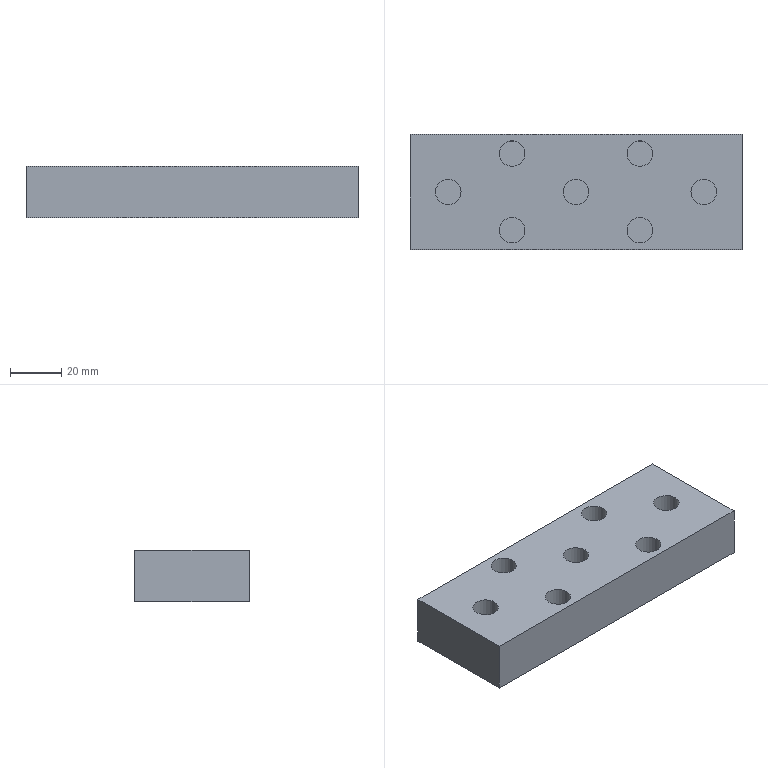NC program | NX | posted with a generic post | part box 130 x 45 x 20 mm
Lines 288 to 1135 of 3690:
(PLANAR_MILL_1 , TOOL : D8开粗)
N556 T09 M6
N558 G54
N560 G17 G0 G90 X-25.452 Y14.224 S4500 M3
N562 G43 Z30. H9
N564 Z1.
N566 G94 G1 X-25.239 Y14.101 Z0.987 F800.
N568 X-24.753 Y14.103 Z0.962
N570 X-24.347 Y14.338 Z0.937
N572 X-24.1 Y14.766 Z0.911
N574 Y15.234 Z0.887
N576 X-24.347 Y15.662 Z0.861
N578 X-24.753 Y15.897 Z0.836
N580 X-25.239 Y15.899 Z0.811
N582 X-25.659 Y15.656 Z0.785
N584 X-25.9 Y15.234 Z0.76
N586 Y14.766 Z0.735
N588 X-25.659 Y14.344 Z0.71
N590 X-25.239 Y14.101 Z0.684
N592 X-24.753 Y14.103 Z0.659
N594 X-24.347 Y14.338 Z0.634
N596 X-24.1 Y14.766 Z0.608
N598 Y15.234 Z0.584
N600 X-24.347 Y15.662 Z0.558
N602 X-24.753 Y15.897 Z0.533
N604 X-25.239 Y15.899 Z0.508
N606 X-25.659 Y15.656 Z0.483
N608 X-25.9 Y15.234 Z0.457
N610 Y14.766 Z0.432
N612 X-25.659 Y14.344 Z0.407
N614 X-25.239 Y14.101 Z0.382
N616 X-24.753 Y14.103 Z0.356
N618 X-24.347 Y14.338 Z0.332
N620 X-24.1 Y14.766 Z0.306
N622 Y15.234 Z0.281
N624 X-24.347 Y15.662 Z0.255
N626 X-24.753 Y15.897 Z0.231
N628 X-25.239 Y15.899 Z0.205
N630 X-25.659 Y15.656 Z0.18
N632 X-25.9 Y15.234 Z0.154
N634 Y14.766 Z0.13
N636 X-25.659 Y14.344 Z0.104
N638 X-25.239 Y14.101 Z0.079
N640 X-24.753 Y14.103 Z0.053
N642 X-24.347 Y14.338 Z0.029
N644 X-24.1 Y14.766 Z0.003
N646 Y15.234 Z-0.022
N648 X-24.347 Y15.662 Z-0.048
N650 X-24.753 Y15.897 Z-0.072
N652 X-25.239 Y15.899 Z-0.098
N654 X-25.659 Y15.656 Z-0.123
N656 X-25.9 Y15.234 Z-0.148
N658 Y14.766 Z-0.173
N660 X-25.659 Y14.344 Z-0.198
N662 X-25.239 Y14.101 Z-0.224
N664 X-24.753 Y14.103 Z-0.249
N666 X-24.347 Y14.338 Z-0.274
N668 X-24.1 Y14.766 Z-0.3
N670 Y15.234 Z-0.324
N672 X-24.347 Y15.662 Z-0.35
N674 X-24.753 Y15.897 Z-0.375
N676 X-25.239 Y15.899 Z-0.4
N678 X-25.659 Y15.656 Z-0.426
N680 X-25.9 Y15.234 Z-0.451
N682 Y14.766 Z-0.476
N684 X-25.659 Y14.344 Z-0.501
N686 X-25.239 Y14.101 Z-0.527
N688 X-24.753 Y14.103 Z-0.552
N690 X-24.347 Y14.338 Z-0.577
N692 X-24.1 Y14.766 Z-0.603
N694 Y15.234 Z-0.627
N696 X-24.347 Y15.662 Z-0.653
N698 X-24.753 Y15.897 Z-0.678
N700 X-25.239 Y15.899 Z-0.703
N702 X-25.659 Y15.656 Z-0.728
N704 X-25.9 Y15.234 Z-0.754
N706 Y14.766 Z-0.778
N708 X-25.659 Y14.344 Z-0.804
N710 X-25.239 Y14.101 Z-0.829
N712 X-24.753 Y14.103 Z-0.855
N714 X-24.347 Y14.338 Z-0.879
N716 X-24.1 Y14.766 Z-0.905
N718 Y15.234 Z-0.93
N720 X-24.347 Y15.662 Z-0.956
N722 X-24.753 Y15.897 Z-0.98
N724 X-25.239 Y15.899 Z-1.006
N726 X-25.659 Y15.656 Z-1.031
N728 X-25.9 Y15.234 Z-1.057
N730 Y14.766 Z-1.081
N732 X-25.659 Y14.344 Z-1.107
N734 X-25.239 Y14.101 Z-1.132
N736 X-24.753 Y14.103 Z-1.158
N738 X-24.347 Y14.338 Z-1.182
N740 X-24.1 Y14.766 Z-1.208
N742 Y15.234 Z-1.233
N744 X-24.347 Y15.662 Z-1.259
N746 X-24.753 Y15.897 Z-1.283
N748 X-25.239 Y15.899 Z-1.309
N750 X-25.659 Y15.656 Z-1.334
N752 X-25.9 Y15.234 Z-1.359
N754 Y14.766 Z-1.384
N756 X-25.659 Y14.344 Z-1.409
N758 X-25.239 Y14.101 Z-1.435
N760 X-24.753 Y14.103 Z-1.46
N762 X-24.347 Y14.338 Z-1.485
N764 X-24.1 Y14.766 Z-1.511
N766 Y15.234 Z-1.535
N768 X-24.347 Y15.662 Z-1.561
N770 X-24.753 Y15.897 Z-1.586
N772 X-25.239 Y15.899 Z-1.611
N774 X-25.659 Y15.656 Z-1.637
N776 X-25.9 Y15.234 Z-1.662
N778 Y14.766 Z-1.687
N780 X-25.659 Y14.344 Z-1.712
N782 X-25.239 Y14.101 Z-1.738
N784 X-24.753 Y14.103 Z-1.763
N786 X-24.347 Y14.338 Z-1.788
N788 X-24.1 Y14.766 Z-1.814
N790 Y15.234 Z-1.838
N792 X-24.347 Y15.662 Z-1.864
N794 X-24.753 Y15.897 Z-1.889
N796 X-25.239 Y15.899 Z-1.914
N798 X-25.659 Y15.656 Z-1.939
N800 X-25.9 Y15.234 Z-1.965
N802 Y14.766 Z-1.989
N804 X-25.659 Y14.344 Z-2.015
N806 X-25.239 Y14.101 Z-2.04
N808 X-24.753 Y14.103 Z-2.066
N810 X-24.347 Y14.338 Z-2.09
N812 X-24.1 Y14.766 Z-2.116
N814 Y15.234 Z-2.141
N816 X-24.347 Y15.662 Z-2.167
N818 X-24.753 Y15.897 Z-2.191
N820 X-25.239 Y15.899 Z-2.217
N822 X-25.659 Y15.656 Z-2.242
N824 X-25.9 Y15.234 Z-2.268
N826 Y14.766 Z-2.292
N828 X-25.659 Y14.344 Z-2.318
N830 X-25.239 Y14.101 Z-2.343
N832 X-24.753 Y14.103 Z-2.369
N834 X-24.347 Y14.338 Z-2.393
N836 X-24.1 Y14.766 Z-2.419
N838 Y15.234 Z-2.444
N840 X-24.347 Y15.662 Z-2.469
N842 X-24.753 Y15.897 Z-2.494
N844 X-25.239 Y15.899 Z-2.52
N846 X-25.659 Y15.656 Z-2.545
N848 X-25.9 Y15.234 Z-2.57
N850 Y14.766 Z-2.595
N852 X-25.659 Y14.344 Z-2.62
N854 X-25.239 Y14.101 Z-2.646
N856 X-24.753 Y14.103 Z-2.671
N858 X-24.347 Y14.338 Z-2.696
N860 X-24.1 Y14.766 Z-2.722
N862 Y15.234 Z-2.746
N864 X-24.347 Y15.662 Z-2.772
N866 X-24.753 Y15.897 Z-2.797
N868 X-25.239 Y15.899 Z-2.822
N870 X-25.659 Y15.656 Z-2.848
N872 X-25.9 Y15.234 Z-2.873
N874 Y14.766 Z-2.898
N876 X-25.659 Y14.344 Z-2.923
N878 X-25.239 Y14.101 Z-2.949
N880 X-24.753 Y14.103 Z-2.974
N882 X-24.347 Y14.338 Z-2.999
N884 X-24.1 Y14.766 Z-3.025
N886 Y15.234 Z-3.049
N888 X-24.347 Y15.662 Z-3.075
N890 X-24.753 Y15.897 Z-3.1
N892 X-25.239 Y15.899 Z-3.125
N894 X-25.659 Y15.656 Z-3.15
N896 X-25.9 Y15.234 Z-3.176
N898 Y14.766 Z-3.2
N900 X-25.659 Y14.344 Z-3.226
N902 X-25.239 Y14.101 Z-3.251
N904 X-24.753 Y14.103 Z-3.277
N906 X-24.347 Y14.338 Z-3.301
N908 X-24.1 Y14.766 Z-3.327
N910 Y15.234 Z-3.352
N912 X-24.347 Y15.662 Z-3.378
N914 X-24.753 Y15.897 Z-3.402
N916 X-25.239 Y15.899 Z-3.428
N918 X-25.659 Y15.656 Z-3.453
N920 X-25.9 Y15.234 Z-3.479
N922 Y14.766 Z-3.503
N924 X-25.659 Y14.344 Z-3.529
N926 X-25.239 Y14.101 Z-3.554
N928 X-24.753 Y14.103 Z-3.58
N930 X-24.347 Y14.338 Z-3.604
N932 X-24.1 Y14.766 Z-3.63
N934 Y15.234 Z-3.655
N936 X-24.347 Y15.662 Z-3.68
N938 X-24.753 Y15.897 Z-3.705
N940 X-25.239 Y15.899 Z-3.73
N942 X-25.659 Y15.656 Z-3.756
N944 X-25.9 Y15.234 Z-3.781
N946 Y14.766 Z-3.806
N948 X-25.659 Y14.344 Z-3.831
N950 X-25.239 Y14.101 Z-3.857
N952 X-24.753 Y14.103 Z-3.882
N954 X-24.347 Y14.338 Z-3.907
N956 X-24.1 Y14.766 Z-3.933
N958 Y15.234 Z-3.957
N960 X-24.347 Y15.662 Z-3.983
N962 X-24.753 Y15.897 Z-4.008
N964 X-25.239 Y15.899 Z-4.033
N966 X-25.659 Y15.656 Z-4.059
N968 X-25.9 Y15.234 Z-4.084
N970 Y14.766 Z-4.109
N972 X-25.659 Y14.344 Z-4.134
N974 X-25.239 Y14.101 Z-4.16
N976 X-24.753 Y14.103 Z-4.185
N978 X-24.347 Y14.338 Z-4.21
N980 X-24.1 Y14.766 Z-4.236
N982 Y15.234 Z-4.26
N984 X-24.347 Y15.662 Z-4.286
N986 X-24.753 Y15.897 Z-4.311
N988 X-25.239 Y15.899 Z-4.336
N990 X-25.659 Y15.656 Z-4.361
N992 X-25.9 Y15.234 Z-4.387
N994 Y14.766 Z-4.411
N996 X-25.659 Y14.344 Z-4.437
N998 X-25.239 Y14.101 Z-4.462
N1000 X-24.753 Y14.103 Z-4.488
N1002 X-24.347 Y14.338 Z-4.512
N1004 X-24.1 Y14.766 Z-4.538
N1006 Y15.234 Z-4.563
N1008 X-24.347 Y15.662 Z-4.589
N1010 X-24.753 Y15.897 Z-4.613
N1012 X-25.239 Y15.899 Z-4.639
N1014 X-25.659 Y15.656 Z-4.664
N1016 X-25.9 Y15.234 Z-4.69
N1018 Y14.766 Z-4.714
N1020 X-25.659 Y14.344 Z-4.74
N1022 X-25.239 Y14.101 Z-4.765
N1024 X-24.753 Y14.103 Z-4.791
N1026 X-24.347 Y14.338 Z-4.815
N1028 X-24.1 Y14.766 Z-4.841
N1030 Y15.234 Z-4.866
N1032 X-24.347 Y15.662 Z-4.891
N1034 X-24.753 Y15.897 Z-4.916
N1036 X-25.239 Y15.899 Z-4.941
N1038 X-25.659 Y15.656 Z-4.967
N1040 X-25.9 Y15.234 Z-4.992
N1042 Y14.766 Z-5.017
N1044 X-25.659 Y14.344 Z-5.042
N1046 X-25.239 Y14.101 Z-5.068
N1048 X-24.753 Y14.103 Z-5.093
N1050 X-24.347 Y14.338 Z-5.118
N1052 X-24.1 Y14.766 Z-5.144
N1054 Y15.234 Z-5.168
N1056 X-24.347 Y15.662 Z-5.194
N1058 X-24.753 Y15.897 Z-5.219
N1060 X-25.239 Y15.899 Z-5.244
N1062 X-25.659 Y15.656 Z-5.27
N1064 X-25.9 Y15.234 Z-5.295
N1066 Y14.766 Z-5.32
N1068 X-25.659 Y14.344 Z-5.345
N1070 X-25.239 Y14.101 Z-5.371
N1072 X-24.753 Y14.103 Z-5.396
N1074 X-24.347 Y14.338 Z-5.421
N1076 X-24.1 Y14.766 Z-5.447
N1078 Y15.234 Z-5.471
N1080 X-24.347 Y15.662 Z-5.497
N1082 X-24.753 Y15.897 Z-5.522
N1084 X-25.239 Y15.899 Z-5.547
N1086 X-25.659 Y15.656 Z-5.572
N1088 X-25.9 Y15.234 Z-5.598
N1090 Y14.766 Z-5.622
N1092 X-25.659 Y14.344 Z-5.648
N1094 X-25.239 Y14.101 Z-5.673
N1096 X-24.753 Y14.103 Z-5.699
N1098 X-24.347 Y14.338 Z-5.723
N1100 X-24.1 Y14.766 Z-5.749
N1102 Y15.234 Z-5.774
N1104 X-24.347 Y15.662 Z-5.8
N1106 X-24.753 Y15.897 Z-5.824
N1108 X-25.239 Y15.899 Z-5.85
N1110 X-25.659 Y15.656 Z-5.875
N1112 X-25.9 Y15.234 Z-5.901
N1114 Y14.766 Z-5.925
N1116 X-25.659 Y14.344 Z-5.951
N1118 X-25.239 Y14.101 Z-5.976
N1120 X-24.753 Y14.103 Z-6.002
N1122 X-24.347 Y14.338 Z-6.026
N1124 X-24.1 Y14.766 Z-6.052
N1126 Y15.234 Z-6.077
N1128 X-24.347 Y15.662 Z-6.102
N1130 X-24.753 Y15.897 Z-6.127
N1132 X-25.239 Y15.899 Z-6.152
N1134 X-25.659 Y15.656 Z-6.178
N1136 X-25.9 Y15.234 Z-6.203
N1138 Y14.766 Z-6.228
N1140 X-25.659 Y14.344 Z-6.253
N1142 X-25.239 Y14.101 Z-6.279
N1144 X-24.753 Y14.103 Z-6.304
N1146 X-24.347 Y14.338 Z-6.329
N1148 X-24.1 Y14.766 Z-6.355
N1150 Y15.234 Z-6.379
N1152 X-24.347 Y15.662 Z-6.405
N1154 X-24.753 Y15.897 Z-6.43
N1156 X-25.239 Y15.899 Z-6.455
N1158 X-25.659 Y15.656 Z-6.481
N1160 X-25.9 Y15.234 Z-6.506
N1162 Y14.766 Z-6.531
N1164 X-25.659 Y14.344 Z-6.556
N1166 X-25.239 Y14.101 Z-6.582
N1168 X-24.753 Y14.103 Z-6.607
N1170 X-24.347 Y14.338 Z-6.632
N1172 X-24.1 Y14.766 Z-6.658
N1174 Y15.234 Z-6.682
N1176 X-24.347 Y15.662 Z-6.708
N1178 X-24.753 Y15.897 Z-6.733
N1180 X-25.239 Y15.899 Z-6.758
N1182 X-25.659 Y15.656 Z-6.783
N1184 X-25.9 Y15.234 Z-6.809
N1186 Y14.766 Z-6.833
N1188 X-25.659 Y14.344 Z-6.859
N1190 X-25.239 Y14.101 Z-6.884
N1192 X-24.753 Y14.103 Z-6.91
N1194 X-24.347 Y14.338 Z-6.934
N1196 X-24.1 Y14.766 Z-6.96
N1198 Y15.234 Z-6.985
N1200 X-24.347 Y15.662 Z-7.011
N1202 X-24.753 Y15.897 Z-7.035
N1204 X-25.239 Y15.899 Z-7.061
N1206 X-25.659 Y15.656 Z-7.086
N1208 X-25.9 Y15.234 Z-7.112
N1210 Y14.766 Z-7.136
N1212 X-25.659 Y14.344 Z-7.162
N1214 X-25.239 Y14.101 Z-7.187
N1216 X-24.753 Y14.103 Z-7.213
N1218 X-24.347 Y14.338 Z-7.237
N1220 X-24.1 Y14.766 Z-7.263
N1222 Y15.234 Z-7.288
N1224 X-24.347 Y15.662 Z-7.313
N1226 X-24.753 Y15.897 Z-7.338
N1228 X-25.239 Y15.899 Z-7.363
N1230 X-25.659 Y15.656 Z-7.389
N1232 X-25.9 Y15.234 Z-7.414
N1234 Y14.766 Z-7.439
N1236 X-25.659 Y14.344 Z-7.464
N1238 X-25.239 Y14.101 Z-7.49
N1240 X-24.753 Y14.103 Z-7.515
N1242 X-24.347 Y14.338 Z-7.54
N1244 X-24.1 Y14.766 Z-7.566
N1246 Y15.234 Z-7.59
N1248 X-24.347 Y15.662 Z-7.616
N1250 X-24.753 Y15.897 Z-7.641
N1252 X-25.239 Y15.899 Z-7.666
N1254 X-25.659 Y15.656 Z-7.692
N1256 X-25.9 Y15.234 Z-7.717
N1258 Y14.766 Z-7.742
N1260 X-25.659 Y14.344 Z-7.767
N1262 X-25.239 Y14.101 Z-7.793
N1264 X-24.753 Y14.103 Z-7.818
N1266 X-24.347 Y14.338 Z-7.843
N1268 X-24.1 Y14.766 Z-7.868
N1270 Y15.234 Z-7.893
N1272 X-24.347 Y15.662 Z-7.919
N1274 X-24.753 Y15.897 Z-7.944
N1276 X-25.239 Y15.899 Z-7.969
N1278 X-25.659 Y15.656 Z-7.994
N1280 X-25.9 Y15.234 Z-8.02
N1282 Y14.766 Z-8.044
N1284 X-25.659 Y14.344 Z-8.07
N1286 X-25.239 Y14.101 Z-8.095
N1288 X-24.753 Y14.103 Z-8.121
N1290 X-24.347 Y14.338 Z-8.145
N1292 X-24.1 Y14.766 Z-8.171
N1294 Y15.234 Z-8.196
N1296 X-24.347 Y15.662 Z-8.222
N1298 X-24.753 Y15.897 Z-8.246
N1300 X-25.239 Y15.899 Z-8.272
N1302 X-25.659 Y15.656 Z-8.297
N1304 X-25.9 Y15.234 Z-8.323
N1306 Y14.766 Z-8.347
N1308 X-25.659 Y14.344 Z-8.373
N1310 X-25.239 Y14.101 Z-8.398
N1312 X-24.753 Y14.103 Z-8.424
N1314 X-24.347 Y14.338 Z-8.448
N1316 X-24.1 Y14.766 Z-8.474
N1318 Y15.234 Z-8.499
N1320 X-24.347 Y15.662 Z-8.524
N1322 X-24.753 Y15.897 Z-8.549
N1324 X-25.239 Y15.899 Z-8.574
N1326 X-25.659 Y15.656 Z-8.6
N1328 X-25.9 Y15.234 Z-8.625
N1330 Y14.766 Z-8.65
N1332 X-25.659 Y14.344 Z-8.675
N1334 X-25.239 Y14.101 Z-8.701
N1336 X-24.753 Y14.103 Z-8.726
N1338 X-24.347 Y14.338 Z-8.751
N1340 X-24.1 Y14.766 Z-8.777
N1342 Y15.234 Z-8.801
N1344 X-24.347 Y15.662 Z-8.827
N1346 X-24.753 Y15.897 Z-8.852
N1348 X-25.239 Y15.899 Z-8.877
N1350 X-25.659 Y15.656 Z-8.903
N1352 X-25.9 Y15.234 Z-8.928
N1354 Y14.766 Z-8.953
N1356 X-25.659 Y14.344 Z-8.978
N1358 X-25.239 Y14.101 Z-9.004
N1360 X-24.753 Y14.103 Z-9.029
N1362 X-24.347 Y14.338 Z-9.054
N1364 X-24.1 Y14.766 Z-9.079
N1366 Y15.234 Z-9.104
N1368 X-24.347 Y15.662 Z-9.13
N1370 X-24.753 Y15.897 Z-9.154
N1372 X-25.239 Y15.899 Z-9.18
N1374 X-25.659 Y15.656 Z-9.205
N1376 X-25.9 Y15.234 Z-9.231
N1378 Y14.766 Z-9.255
N1380 X-25.659 Y14.344 Z-9.281
N1382 X-25.239 Y14.101 Z-9.306
N1384 X-24.753 Y14.103 Z-9.332
N1386 X-24.347 Y14.338 Z-9.356
N1388 X-24.1 Y14.766 Z-9.382
N1390 Y15.234 Z-9.407
N1392 X-24.347 Y15.662 Z-9.433
N1394 X-24.753 Y15.897 Z-9.457
N1396 X-25.239 Y15.899 Z-9.483
N1398 X-25.659 Y15.656 Z-9.508
N1400 X-25.9 Y15.234 Z-9.534
N1402 Y14.766 Z-9.558
N1404 X-25.659 Y14.344 Z-9.584
N1406 X-25.239 Y14.101 Z-9.609
N1408 X-24.753 Y14.103 Z-9.635
N1410 X-24.347 Y14.338 Z-9.659
N1412 X-24.1 Y14.766 Z-9.685
N1414 Y15.234 Z-9.71
N1416 X-24.347 Y15.662 Z-9.735
N1418 X-24.753 Y15.897 Z-9.76
N1420 X-25.239 Y15.899 Z-9.785
N1422 X-25.659 Y15.656 Z-9.811
N1424 X-25.9 Y15.234 Z-9.836
N1426 Y14.766 Z-9.861
N1428 X-25.659 Y14.344 Z-9.886
N1430 X-25.239 Y14.101 Z-9.912
N1432 X-24.753 Y14.103 Z-9.937
N1434 X-24.347 Y14.338 Z-9.962
N1436 X-24.1 Y14.766 Z-9.988
N1438 Y15. Z-10.
N1440 G3 X-25. Y15.9 R0.9
N1442 X-24.1 Y15. R-0.9
N1444 G1 Z-9.
N1446 G0 Z30.
N1448 X-50.452 Y-0.776
N1450 Z1.
N1452 G1 X-50.239 Y-0.899 Z0.987
N1454 X-49.753 Y-0.897 Z0.962
N1456 X-49.347 Y-0.662 Z0.937
N1458 X-49.1 Y-0.234 Z0.911
N1460 Y0.234 Z0.887
N1462 X-49.347 Y0.662 Z0.861
N1464 X-49.753 Y0.897 Z0.836
N1466 X-50.239 Y0.899 Z0.811
N1468 X-50.659 Y0.656 Z0.785
N1470 X-50.9 Y0.234 Z0.76
N1472 Y-0.234 Z0.735
N1474 X-50.659 Y-0.656 Z0.71
N1476 X-50.239 Y-0.899 Z0.684
N1478 X-49.753 Y-0.897 Z0.659
N1480 X-49.347 Y-0.662 Z0.634
N1482 X-49.1 Y-0.234 Z0.608
N1484 Y0.234 Z0.584
N1486 X-49.347 Y0.662 Z0.558
N1488 X-49.753 Y0.897 Z0.533
N1490 X-50.239 Y0.899 Z0.508
N1492 X-50.659 Y0.656 Z0.483
N1494 X-50.9 Y0.234 Z0.457
N1496 Y-0.234 Z0.432
N1498 X-50.659 Y-0.656 Z0.407
N1500 X-50.239 Y-0.899 Z0.382
N1502 X-49.753 Y-0.897 Z0.356
N1504 X-49.347 Y-0.662 Z0.332
N1506 X-49.1 Y-0.234 Z0.306
N1508 Y0.234 Z0.281
N1510 X-49.347 Y0.662 Z0.255
N1512 X-49.753 Y0.897 Z0.231
N1514 X-50.239 Y0.899 Z0.205
N1516 X-50.659 Y0.656 Z0.18
N1518 X-50.9 Y0.234 Z0.154
N1520 Y-0.234 Z0.13
N1522 X-50.659 Y-0.656 Z0.104
N1524 X-50.239 Y-0.899 Z0.079
N1526 X-49.753 Y-0.897 Z0.053
N1528 X-49.347 Y-0.662 Z0.029
N1530 X-49.1 Y-0.234 Z0.003
N1532 Y0.234 Z-0.022
N1534 X-49.347 Y0.662 Z-0.048
N1536 X-49.753 Y0.897 Z-0.072
N1538 X-50.239 Y0.899 Z-0.098
N1540 X-50.659 Y0.656 Z-0.123
N1542 X-50.9 Y0.234 Z-0.148
N1544 Y-0.234 Z-0.173
N1546 X-50.659 Y-0.656 Z-0.198
N1548 X-50.239 Y-0.899 Z-0.224
N1550 X-49.753 Y-0.897 Z-0.249
N1552 X-49.347 Y-0.662 Z-0.274
N1554 X-49.1 Y-0.234 Z-0.3
N1556 Y0.234 Z-0.324
N1558 X-49.347 Y0.662 Z-0.35
N1560 X-49.753 Y0.897 Z-0.375
N1562 X-50.239 Y0.899 Z-0.4
N1564 X-50.659 Y0.656 Z-0.426
N1566 X-50.9 Y0.234 Z-0.451
N1568 Y-0.234 Z-0.476
N1570 X-50.659 Y-0.656 Z-0.501
N1572 X-50.239 Y-0.899 Z-0.527
N1574 X-49.753 Y-0.897 Z-0.552
N1576 X-49.347 Y-0.662 Z-0.577
N1578 X-49.1 Y-0.234 Z-0.603
N1580 Y0.234 Z-0.627
N1582 X-49.347 Y0.662 Z-0.653
N1584 X-49.753 Y0.897 Z-0.678
N1586 X-50.239 Y0.899 Z-0.703
N1588 X-50.659 Y0.656 Z-0.728
N1590 X-50.9 Y0.234 Z-0.754
N1592 Y-0.234 Z-0.778
N1594 X-50.659 Y-0.656 Z-0.804
N1596 X-50.239 Y-0.899 Z-0.829
N1598 X-49.753 Y-0.897 Z-0.855
N1600 X-49.347 Y-0.662 Z-0.879
N1602 X-49.1 Y-0.234 Z-0.905
N1604 Y0.234 Z-0.93
N1606 X-49.347 Y0.662 Z-0.956
N1608 X-49.753 Y0.897 Z-0.98
N1610 X-50.239 Y0.899 Z-1.006
N1612 X-50.659 Y0.656 Z-1.031
N1614 X-50.9 Y0.234 Z-1.057
N1616 Y-0.234 Z-1.081
N1618 X-50.659 Y-0.656 Z-1.107
N1620 X-50.239 Y-0.899 Z-1.132
N1622 X-49.753 Y-0.897 Z-1.158
N1624 X-49.347 Y-0.662 Z-1.182
N1626 X-49.1 Y-0.234 Z-1.208
N1628 Y0.234 Z-1.233
N1630 X-49.347 Y0.662 Z-1.259
N1632 X-49.753 Y0.897 Z-1.283
N1634 X-50.239 Y0.899 Z-1.309
N1636 X-50.659 Y0.656 Z-1.334
N1638 X-50.9 Y0.234 Z-1.359
N1640 Y-0.234 Z-1.384
N1642 X-50.659 Y-0.656 Z-1.409
N1644 X-50.239 Y-0.899 Z-1.435
N1646 X-49.753 Y-0.897 Z-1.46
N1648 X-49.347 Y-0.662 Z-1.485
N1650 X-49.1 Y-0.234 Z-1.511
N1652 Y0.234 Z-1.535
N1654 X-49.347 Y0.662 Z-1.561
N1656 X-49.753 Y0.897 Z-1.586
N1658 X-50.239 Y0.899 Z-1.611
N1660 X-50.659 Y0.656 Z-1.637
N1662 X-50.9 Y0.234 Z-1.662
N1664 Y-0.234 Z-1.687
N1666 X-50.659 Y-0.656 Z-1.712
N1668 X-50.239 Y-0.899 Z-1.738
N1670 X-49.753 Y-0.897 Z-1.763
N1672 X-49.347 Y-0.662 Z-1.788
N1674 X-49.1 Y-0.234 Z-1.814
N1676 Y0.234 Z-1.838
N1678 X-49.347 Y0.662 Z-1.864
N1680 X-49.753 Y0.897 Z-1.889
N1682 X-50.239 Y0.899 Z-1.914
N1684 X-50.659 Y0.656 Z-1.939
N1686 X-50.9 Y0.234 Z-1.965
N1688 Y-0.234 Z-1.989
N1690 X-50.659 Y-0.656 Z-2.015
N1692 X-50.239 Y-0.899 Z-2.04
N1694 X-49.753 Y-0.897 Z-2.066
N1696 X-49.347 Y-0.662 Z-2.09
N1698 X-49.1 Y-0.234 Z-2.116
N1700 Y0.234 Z-2.141
N1702 X-49.347 Y0.662 Z-2.167
N1704 X-49.753 Y0.897 Z-2.191
N1706 X-50.239 Y0.899 Z-2.217
N1708 X-50.659 Y0.656 Z-2.242
N1710 X-50.9 Y0.234 Z-2.268
N1712 Y-0.234 Z-2.292
N1714 X-50.659 Y-0.656 Z-2.318
N1716 X-50.239 Y-0.899 Z-2.343
N1718 X-49.753 Y-0.897 Z-2.369
N1720 X-49.347 Y-0.662 Z-2.393
N1722 X-49.1 Y-0.234 Z-2.419
N1724 Y0.234 Z-2.444
N1726 X-49.347 Y0.662 Z-2.469
N1728 X-49.753 Y0.897 Z-2.494
N1730 X-50.239 Y0.899 Z-2.52
N1732 X-50.659 Y0.656 Z-2.545
N1734 X-50.9 Y0.234 Z-2.57
N1736 Y-0.234 Z-2.595
N1738 X-50.659 Y-0.656 Z-2.62
N1740 X-50.239 Y-0.899 Z-2.646
N1742 X-49.753 Y-0.897 Z-2.671
N1744 X-49.347 Y-0.662 Z-2.696
N1746 X-49.1 Y-0.234 Z-2.722
N1748 Y0.234 Z-2.746
N1750 X-49.347 Y0.662 Z-2.772
N1752 X-49.753 Y0.897 Z-2.797
N1754 X-50.239 Y0.899 Z-2.822
N1756 X-50.659 Y0.656 Z-2.848
N1758 X-50.9 Y0.234 Z-2.873
N1760 Y-0.234 Z-2.898
N1762 X-50.659 Y-0.656 Z-2.923
N1764 X-50.239 Y-0.899 Z-2.949
N1766 X-49.753 Y-0.897 Z-2.974
N1768 X-49.347 Y-0.662 Z-2.999
N1770 X-49.1 Y-0.234 Z-3.025
N1772 Y0.234 Z-3.049
N1774 X-49.347 Y0.662 Z-3.075
N1776 X-49.753 Y0.897 Z-3.1
N1778 X-50.239 Y0.899 Z-3.125
N1780 X-50.659 Y0.656 Z-3.15
N1782 X-50.9 Y0.234 Z-3.176
N1784 Y-0.234 Z-3.2
N1786 X-50.659 Y-0.656 Z-3.226
N1788 X-50.239 Y-0.899 Z-3.251
N1790 X-49.753 Y-0.897 Z-3.277
N1792 X-49.347 Y-0.662 Z-3.301
N1794 X-49.1 Y-0.234 Z-3.327
N1796 Y0.234 Z-3.352
N1798 X-49.347 Y0.662 Z-3.378
N1800 X-49.753 Y0.897 Z-3.402
N1802 X-50.239 Y0.899 Z-3.428
N1804 X-50.659 Y0.656 Z-3.453
N1806 X-50.9 Y0.234 Z-3.479
N1808 Y-0.234 Z-3.503
N1810 X-50.659 Y-0.656 Z-3.529
N1812 X-50.239 Y-0.899 Z-3.554
N1814 X-49.753 Y-0.897 Z-3.58
N1816 X-49.347 Y-0.662 Z-3.604
N1818 X-49.1 Y-0.234 Z-3.63
N1820 Y0.234 Z-3.655
N1822 X-49.347 Y0.662 Z-3.68
N1824 X-49.753 Y0.897 Z-3.705
N1826 X-50.239 Y0.899 Z-3.73
N1828 X-50.659 Y0.656 Z-3.756
N1830 X-50.9 Y0.234 Z-3.781
N1832 Y-0.234 Z-3.806
N1834 X-50.659 Y-0.656 Z-3.831
N1836 X-50.239 Y-0.899 Z-3.857
N1838 X-49.753 Y-0.897 Z-3.882
N1840 X-49.347 Y-0.662 Z-3.907
N1842 X-49.1 Y-0.234 Z-3.933
N1844 Y0.234 Z-3.957
N1846 X-49.347 Y0.662 Z-3.983
N1848 X-49.753 Y0.897 Z-4.008
N1850 X-50.239 Y0.899 Z-4.033
N1852 X-50.659 Y0.656 Z-4.059
N1854 X-50.9 Y0.234 Z-4.084
N1856 Y-0.234 Z-4.109
N1858 X-50.659 Y-0.656 Z-4.134
N1860 X-50.239 Y-0.899 Z-4.16
N1862 X-49.753 Y-0.897 Z-4.185
N1864 X-49.347 Y-0.662 Z-4.21
N1866 X-49.1 Y-0.234 Z-4.236
N1868 Y0.234 Z-4.26
N1870 X-49.347 Y0.662 Z-4.286
N1872 X-49.753 Y0.897 Z-4.311
N1874 X-50.239 Y0.899 Z-4.336
N1876 X-50.659 Y0.656 Z-4.361
N1878 X-50.9 Y0.234 Z-4.387
N1880 Y-0.234 Z-4.411
N1882 X-50.659 Y-0.656 Z-4.437
N1884 X-50.239 Y-0.899 Z-4.462
N1886 X-49.753 Y-0.897 Z-4.488
N1888 X-49.347 Y-0.662 Z-4.512
N1890 X-49.1 Y-0.234 Z-4.538
N1892 Y0.234 Z-4.563
N1894 X-49.347 Y0.662 Z-4.589
N1896 X-49.753 Y0.897 Z-4.613
N1898 X-50.239 Y0.899 Z-4.639
N1900 X-50.659 Y0.656 Z-4.664
N1902 X-50.9 Y0.234 Z-4.69
N1904 Y-0.234 Z-4.714
N1906 X-50.659 Y-0.656 Z-4.74
N1908 X-50.239 Y-0.899 Z-4.765
N1910 X-49.753 Y-0.897 Z-4.791
N1912 X-49.347 Y-0.662 Z-4.815
N1914 X-49.1 Y-0.234 Z-4.841
N1916 Y0.234 Z-4.866
N1918 X-49.347 Y0.662 Z-4.891
N1920 X-49.753 Y0.897 Z-4.916
N1922 X-50.239 Y0.899 Z-4.941
N1924 X-50.659 Y0.656 Z-4.967
N1926 X-50.9 Y0.234 Z-4.992
N1928 Y-0.234 Z-5.017
N1930 X-50.659 Y-0.656 Z-5.042
N1932 X-50.239 Y-0.899 Z-5.068
N1934 X-49.753 Y-0.897 Z-5.093
N1936 X-49.347 Y-0.662 Z-5.118
N1938 X-49.1 Y-0.234 Z-5.144
N1940 Y0.234 Z-5.168
N1942 X-49.347 Y0.662 Z-5.194
N1944 X-49.753 Y0.897 Z-5.219
N1946 X-50.239 Y0.899 Z-5.244
N1948 X-50.659 Y0.656 Z-5.27
N1950 X-50.9 Y0.234 Z-5.295
N1952 Y-0.234 Z-5.32
N1954 X-50.659 Y-0.656 Z-5.345
N1956 X-50.239 Y-0.899 Z-5.371
N1958 X-49.753 Y-0.897 Z-5.396
N1960 X-49.347 Y-0.662 Z-5.421
N1962 X-49.1 Y-0.234 Z-5.447
N1964 Y0.234 Z-5.471
N1966 X-49.347 Y0.662 Z-5.497
N1968 X-49.753 Y0.897 Z-5.522
N1970 X-50.239 Y0.899 Z-5.547
N1972 X-50.659 Y0.656 Z-5.572
N1974 X-50.9 Y0.234 Z-5.598
N1976 Y-0.234 Z-5.622
N1978 X-50.659 Y-0.656 Z-5.648
N1980 X-50.239 Y-0.899 Z-5.673
N1982 X-49.753 Y-0.897 Z-5.699
N1984 X-49.347 Y-0.662 Z-5.723
N1986 X-49.1 Y-0.234 Z-5.749
N1988 Y0.234 Z-5.774
N1990 X-49.347 Y0.662 Z-5.8
N1992 X-49.753 Y0.897 Z-5.824
N1994 X-50.239 Y0.899 Z-5.85
N1996 X-50.659 Y0.656 Z-5.875
N1998 X-50.9 Y0.234 Z-5.901
N2000 Y-0.234 Z-5.925
N2002 X-50.659 Y-0.656 Z-5.951
N2004 X-50.239 Y-0.899 Z-5.976
N2006 X-49.753 Y-0.897 Z-6.002
N2008 X-49.347 Y-0.662 Z-6.026
N2010 X-49.1 Y-0.234 Z-6.052
N2012 Y0.234 Z-6.077
N2014 X-49.347 Y0.662 Z-6.102
N2016 X-49.753 Y0.897 Z-6.127
N2018 X-50.239 Y0.899 Z-6.152
N2020 X-50.659 Y0.656 Z-6.178
N2022 X-50.9 Y0.234 Z-6.203
N2024 Y-0.234 Z-6.228
N2026 X-50.659 Y-0.656 Z-6.253
N2028 X-50.239 Y-0.899 Z-6.279
N2030 X-49.753 Y-0.897 Z-6.304
N2032 X-49.347 Y-0.662 Z-6.329
N2034 X-49.1 Y-0.234 Z-6.355
N2036 Y0.234 Z-6.379
N2038 X-49.347 Y0.662 Z-6.405
N2040 X-49.753 Y0.897 Z-6.43
N2042 X-50.239 Y0.899 Z-6.455
N2044 X-50.659 Y0.656 Z-6.481
N2046 X-50.9 Y0.234 Z-6.506
N2048 Y-0.234 Z-6.531
N2050 X-50.659 Y-0.656 Z-6.556
N2052 X-50.239 Y-0.899 Z-6.582
N2054 X-49.753 Y-0.897 Z-6.607
N2056 X-49.347 Y-0.662 Z-6.632
N2058 X-49.1 Y-0.234 Z-6.658
N2060 Y0.234 Z-6.682
N2062 X-49.347 Y0.662 Z-6.708
N2064 X-49.753 Y0.897 Z-6.733
N2066 X-50.239 Y0.899 Z-6.758
N2068 X-50.659 Y0.656 Z-6.783
N2070 X-50.9 Y0.234 Z-6.809
N2072 Y-0.234 Z-6.833
N2074 X-50.659 Y-0.656 Z-6.859
N2076 X-50.239 Y-0.899 Z-6.884
N2078 X-49.753 Y-0.897 Z-6.91
N2080 X-49.347 Y-0.662 Z-6.934
N2082 X-49.1 Y-0.234 Z-6.96
N2084 Y0.234 Z-6.985
N2086 X-49.347 Y0.662 Z-7.011
N2088 X-49.753 Y0.897 Z-7.035
N2090 X-50.239 Y0.899 Z-7.061
N2092 X-50.659 Y0.656 Z-7.086
N2094 X-50.9 Y0.234 Z-7.112
N2096 Y-0.234 Z-7.136
N2098 X-50.659 Y-0.656 Z-7.162
N2100 X-50.239 Y-0.899 Z-7.187
N2102 X-49.753 Y-0.897 Z-7.213
N2104 X-49.347 Y-0.662 Z-7.237
N2106 X-49.1 Y-0.234 Z-7.263
N2108 Y0.234 Z-7.288
N2110 X-49.347 Y0.662 Z-7.313
N2112 X-49.753 Y0.897 Z-7.338
N2114 X-50.239 Y0.899 Z-7.363
N2116 X-50.659 Y0.656 Z-7.389
N2118 X-50.9 Y0.234 Z-7.414
N2120 Y-0.234 Z-7.439
N2122 X-50.659 Y-0.656 Z-7.464
N2124 X-50.239 Y-0.899 Z-7.49
N2126 X-49.753 Y-0.897 Z-7.515
N2128 X-49.347 Y-0.662 Z-7.54
N2130 X-49.1 Y-0.234 Z-7.566
N2132 Y0.234 Z-7.59
N2134 X-49.347 Y0.662 Z-7.616
N2136 X-49.753 Y0.897 Z-7.641
N2138 X-50.239 Y0.899 Z-7.666
N2140 X-50.659 Y0.656 Z-7.692
N2142 X-50.9 Y0.234 Z-7.717
N2144 Y-0.234 Z-7.742
N2146 X-50.659 Y-0.656 Z-7.767
N2148 X-50.239 Y-0.899 Z-7.793
N2150 X-49.753 Y-0.897 Z-7.818
N2152 X-49.347 Y-0.662 Z-7.843
N2154 X-49.1 Y-0.234 Z-7.868
N2156 Y0.234 Z-7.893
N2158 X-49.347 Y0.662 Z-7.919
N2160 X-49.753 Y0.897 Z-7.944
N2162 X-50.239 Y0.899 Z-7.969
N2164 X-50.659 Y0.656 Z-7.994
N2166 X-50.9 Y0.234 Z-8.02
N2168 Y-0.234 Z-8.044
N2170 X-50.659 Y-0.656 Z-8.07
N2172 X-50.239 Y-0.899 Z-8.095
N2174 X-49.753 Y-0.897 Z-8.121
N2176 X-49.347 Y-0.662 Z-8.145
N2178 X-49.1 Y-0.234 Z-8.171
N2180 Y0.234 Z-8.196
N2182 X-49.347 Y0.662 Z-8.222
N2184 X-49.753 Y0.897 Z-8.246
N2186 X-50.239 Y0.899 Z-8.272
N2188 X-50.659 Y0.656 Z-8.297
N2190 X-50.9 Y0.234 Z-8.323
N2192 Y-0.234 Z-8.347
N2194 X-50.659 Y-0.656 Z-8.373
N2196 X-50.239 Y-0.899 Z-8.398
N2198 X-49.753 Y-0.897 Z-8.424
N2200 X-49.347 Y-0.662 Z-8.448
N2202 X-49.1 Y-0.234 Z-8.474
N2204 Y0.234 Z-8.499
N2206 X-49.347 Y0.662 Z-8.524
N2208 X-49.753 Y0.897 Z-8.549
N2210 X-50.239 Y0.899 Z-8.574
N2212 X-50.659 Y0.656 Z-8.6
N2214 X-50.9 Y0.234 Z-8.625
N2216 Y-0.234 Z-8.65
N2218 X-50.659 Y-0.656 Z-8.675
N2220 X-50.239 Y-0.899 Z-8.701
N2222 X-49.753 Y-0.897 Z-8.726
N2224 X-49.347 Y-0.662 Z-8.751
N2226 X-49.1 Y-0.234 Z-8.777
N2228 Y0.234 Z-8.801
N2230 X-49.347 Y0.662 Z-8.827
N2232 X-49.753 Y0.897 Z-8.852
N2234 X-50.239 Y0.899 Z-8.877
N2236 X-50.659 Y0.656 Z-8.903
N2238 X-50.9 Y0.234 Z-8.928
N2240 Y-0.234 Z-8.953
N2242 X-50.659 Y-0.656 Z-8.978
N2244 X-50.239 Y-0.899 Z-9.004